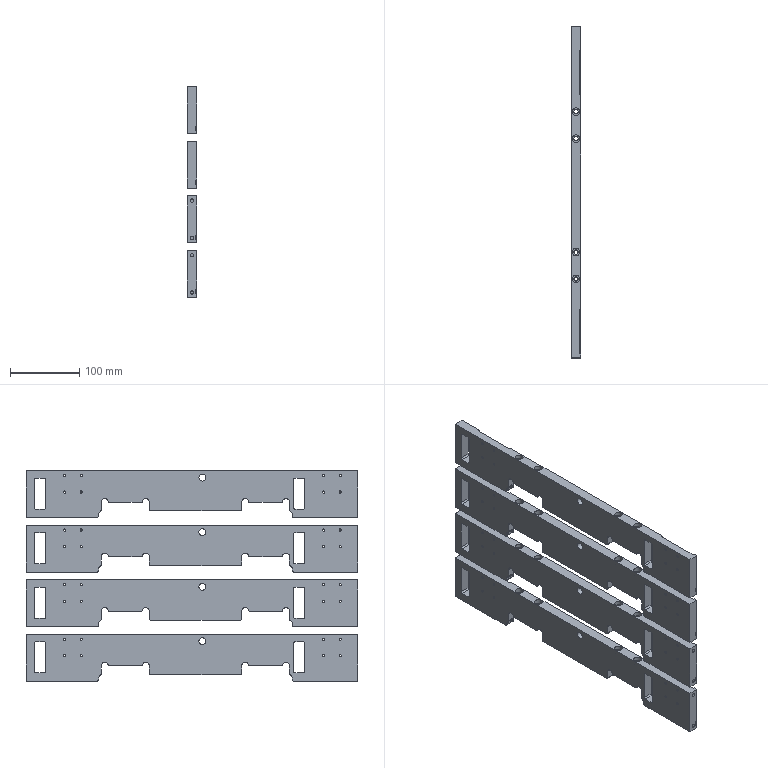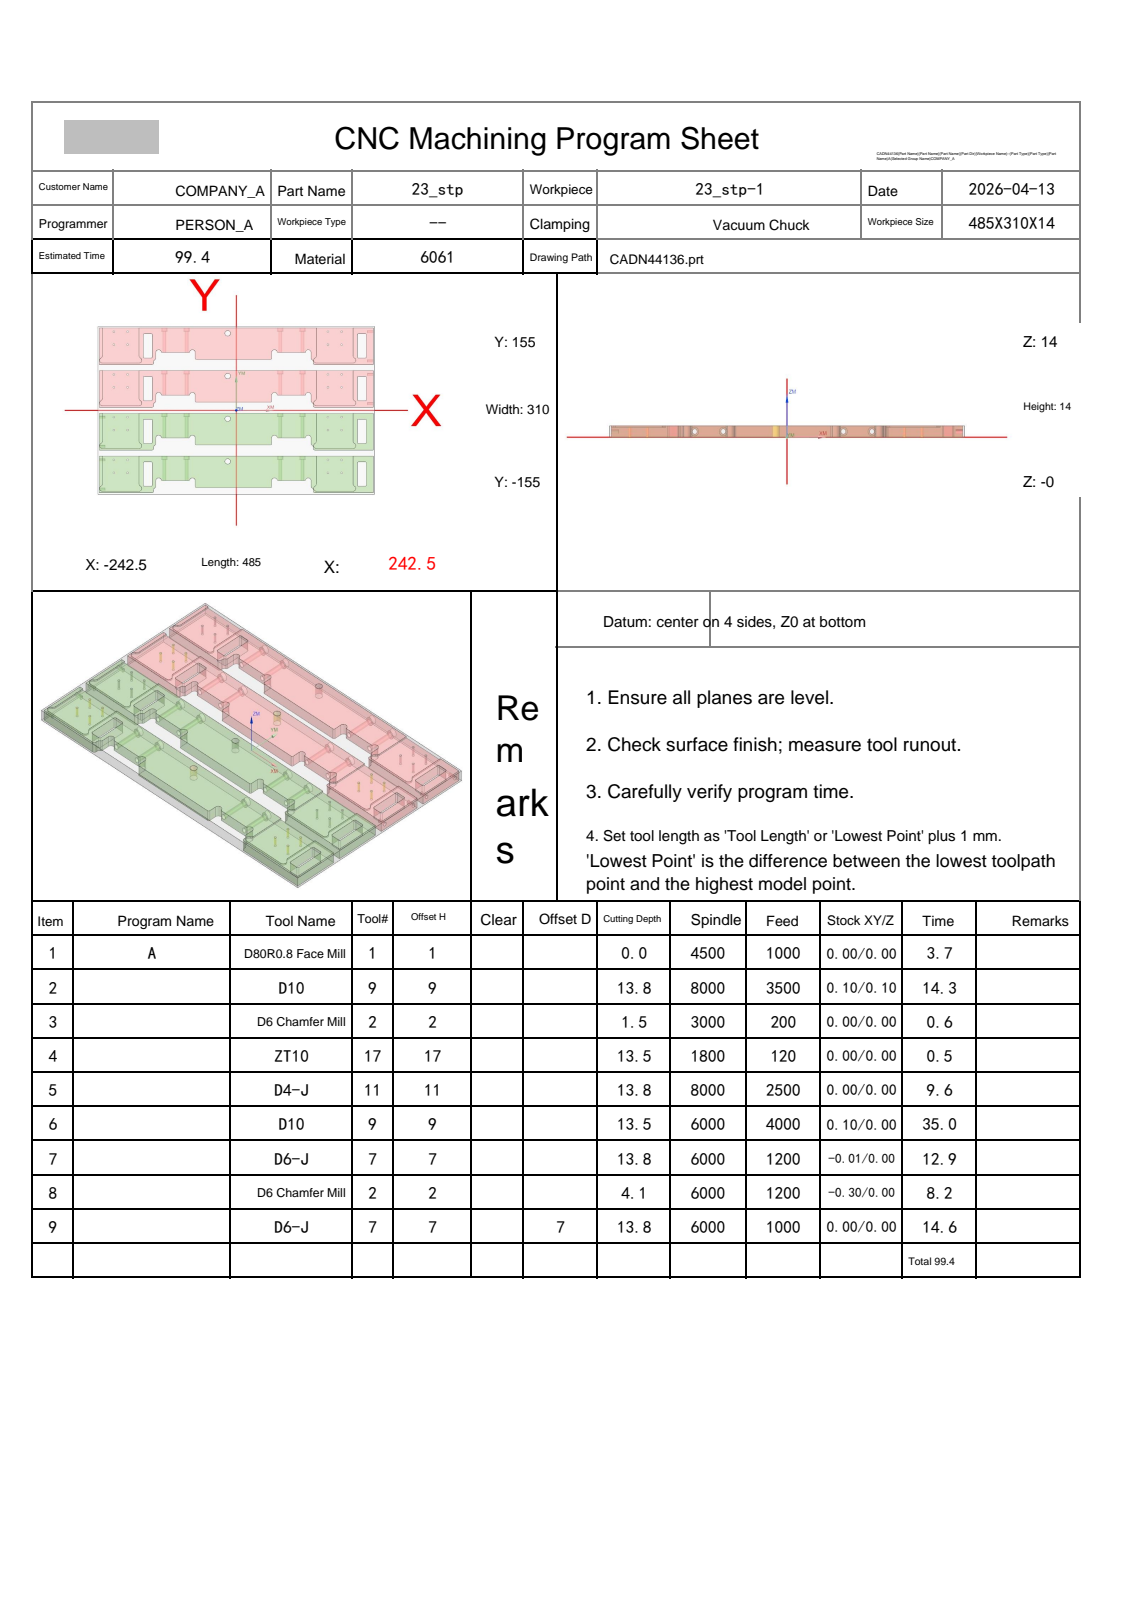NC program | NX | posted by the shop | part box 14 x 480 x 305 mm
Lines 49519 to 51894 of 51894, first 2165 of 2376 lines:
N7 T07 M06
(D6-J  D=6. R=0. H=07 ce=0.30 di=0.00)
G00 G90 G54 X143.75 Y-98.104 M03 S6000
G43 H07 Z34.
M08
Z13.5
G01 Y-83.9 Z13.004 F1200.
X172.5 Z12.
X201.25
Y-135.84
G03 X205.375 Y-142.984 I8.25 J0.0
G02 X206.25 Y-144.5 I-.875 J-1.516
X204.5 Y-146.25 I-1.75 J0.0
G01 X140.5
G02 X138.75 Y-144.5 I0.0 J1.75
X139.625 Y-142.984 I1.75 J0.0
G03 X143.75 Y-135.84 I-4.125 J7.145
G01 Y-83.9
X172.5
Y-88.1
X197.05
Y-135.84
G03 X198.709 Y-142.05 I12.45 J0.0
G01 X146.291
G03 X147.95 Y-135.84 I-10.791 J6.21
G01 Y-88.1
X172.5
Y-92.3
X192.85
Y-135.84
G03 X192.972 Y-137.85 I16.65 J0.0
G01 X152.028
G03 X152.15 Y-135.84 I-16.528 J2.01
G01 Y-92.3
X172.5
Y-96.5
X188.65
Y-133.65
X156.35
Y-96.5
X172.5
Y-100.7
X184.45
Y-129.45
X160.55
Y-100.7
X172.5
Y-104.9
X180.25
Y-125.25
X164.75
Y-104.9
X172.5
Y-109.1
X176.05
Y-121.05
X168.95
Y-109.1
X172.5
Y-111.8
X173.35
Y-118.35
X171.65
Y-111.8
X172.5
X173.
Y-108.2
Z12.5
G00 Z34.
X143.75 Y-19.104
Z13.5
G01 Y-4.9 Z13.004
X172.5 Z12.
X201.25
Y-56.84
G03 X205.375 Y-63.984 I8.25 J0.0
G02 X206.25 Y-65.5 I-.875 J-1.516
X204.5 Y-67.25 I-1.75 J0.0
G01 X140.5
G02 X138.75 Y-65.5 I0.0 J1.75
X139.625 Y-63.984 I1.75 J0.0
G03 X143.75 Y-56.84 I-4.125 J7.145
G01 Y-4.9
X172.5
Y-9.1
X197.05
Y-56.84
G03 X198.709 Y-63.05 I12.45 J0.0
G01 X146.291
G03 X147.95 Y-56.84 I-10.791 J6.21
G01 Y-9.1
X172.5
Y-13.3
X192.85
Y-56.84
G03 X192.972 Y-58.85 I16.65 J0.0
G01 X152.028
G03 X152.15 Y-56.84 I-16.528 J2.01
G01 Y-13.3
X172.5
Y-17.5
X188.65
Y-54.65
X156.35
Y-17.5
X172.5
Y-21.7
X184.45
Y-50.45
X160.55
Y-21.7
X172.5
Y-25.9
X180.25
Y-46.25
X164.75
Y-25.9
X172.5
Y-30.1
X176.05
Y-42.05
X168.95
Y-30.1
X172.5
Y-32.8
X173.35
Y-39.35
X171.65
Y-32.8
X172.5
X173.
Y-29.2
Z12.5
G00 Z34.
X143.75 Y59.896
Z13.5
G01 Y74.1 Z13.004
X172.5 Z12.
X201.25
Y22.16
G03 X205.375 Y15.016 I8.25 J0.0
G02 X206.25 Y13.5 I-.875 J-1.516
X204.5 Y11.75 I-1.75 J0.0
G01 X140.5
G02 X138.75 Y13.5 I0.0 J1.75
X139.625 Y15.016 I1.75 J0.0
G03 X143.75 Y22.16 I-4.125 J7.145
G01 Y74.1
X172.5
Y69.9
X197.05
Y22.16
G03 X198.709 Y15.95 I12.45 J0.0
G01 X146.291
G03 X147.95 Y22.16 I-10.791 J6.21
G01 Y69.9
X172.5
Y65.7
X192.85
Y22.16
G03 X192.972 Y20.15 I16.65 J0.0
G01 X152.028
G03 X152.15 Y22.16 I-16.528 J2.01
G01 Y65.7
X172.5
Y61.5
X188.65
Y24.35
X156.35
Y61.5
X172.5
Y57.3
X184.45
Y28.55
X160.55
Y57.3
X172.5
Y53.1
X180.25
Y32.75
X164.75
Y53.1
X172.5
Y48.9
X176.05
Y36.95
X168.95
Y48.9
X172.5
Y46.2
X173.35
Y39.65
X171.65
Y46.2
X172.5
X173.
Y49.8
Z12.5
G00 Z34.
X172.5 Y158.5
Z12.5
G01 Z12.
Y153.1
X201.25
Y101.16
G03 X205.375 Y94.016 I8.25 J0.0
G02 X206.25 Y92.5 I-.875 J-1.516
X204.5 Y90.75 I-1.75 J0.0
G01 X140.5
G02 X138.75 Y92.5 I0.0 J1.75
X139.625 Y94.016 I1.75 J0.0
G03 X143.75 Y101.16 I-4.125 J7.145
G01 Y153.1
X172.5
Y148.9
X197.05
Y101.16
G03 X198.709 Y94.95 I12.45 J0.0
G01 X146.291
G03 X147.95 Y101.16 I-10.791 J6.21
G01 Y148.9
X172.5
Y144.7
X192.85
Y101.16
G03 X192.972 Y99.15 I16.65 J0.0
G01 X152.028
G03 X152.15 Y101.16 I-16.528 J2.01
G01 Y144.7
X172.5
Y140.5
X188.65
Y103.35
X156.35
Y140.5
X172.5
Y136.3
X184.45
Y107.55
X160.55
Y136.3
X172.5
Y132.1
X180.25
Y111.75
X164.75
Y132.1
X172.5
Y127.9
X176.05
Y115.95
X168.95
Y127.9
X172.5
Y125.2
X173.35
Y118.65
X171.65
Y125.2
X172.5
X173.
Y128.8
Z12.5
G00 Z34.
X-202.5 Y158.5
Z12.5
G01 Z12.
Y153.1
X-173.75
Y101.16
G03 X-169.625 Y94.016 I8.25 J0.0
G02 X-168.75 Y92.5 I-.875 J-1.516
X-170.5 Y90.75 I-1.75 J0.0
G01 X-234.5
G02 X-236.25 Y92.5 I0.0 J1.75
X-235.375 Y94.016 I1.75 J0.0
G03 X-231.25 Y101.16 I-4.125 J7.145
G01 Y153.1
X-202.5
Y148.9
X-177.95
Y101.16
G03 X-176.291 Y94.95 I12.45 J0.0
G01 X-228.709
G03 X-227.05 Y101.16 I-10.791 J6.21
G01 Y148.9
X-202.5
Y144.7
X-182.15
Y101.16
G03 X-182.028 Y99.15 I16.65 J0.0
G01 X-222.972
G03 X-222.85 Y101.16 I-16.528 J2.01
G01 Y144.7
X-202.5
Y140.5
X-186.35
Y103.35
X-218.65
Y140.5
X-202.5
Y136.3
X-190.55
Y107.55
X-214.45
Y136.3
X-202.5
Y132.1
X-194.75
Y111.75
X-210.25
Y132.1
X-202.5
Y127.9
X-198.95
Y115.95
X-206.05
Y127.9
X-202.5
Y125.2
X-201.65
Y118.65
X-203.35
Y125.2
X-202.5
X-202.
Y128.8
Z12.5
G00 Z34.
X-231.25 Y59.896
Z13.5
G01 Y74.1 Z13.004
X-202.5 Z12.
X-173.75
Y22.16
G03 X-169.625 Y15.016 I8.25 J0.0
G02 X-168.75 Y13.5 I-.875 J-1.516
X-170.5 Y11.75 I-1.75 J0.0
G01 X-234.5
G02 X-236.25 Y13.5 I0.0 J1.75
X-235.375 Y15.016 I1.75 J0.0
G03 X-231.25 Y22.16 I-4.125 J7.145
G01 Y74.1
X-202.5
Y69.9
X-177.95
Y22.16
G03 X-176.291 Y15.95 I12.45 J0.0
G01 X-228.709
G03 X-227.05 Y22.16 I-10.791 J6.21
G01 Y69.9
X-202.5
Y65.7
X-182.15
Y22.16
G03 X-182.028 Y20.15 I16.65 J0.0
G01 X-222.972
G03 X-222.85 Y22.16 I-16.528 J2.01
G01 Y65.7
X-202.5
Y61.5
X-186.35
Y24.35
X-218.65
Y61.5
X-202.5
Y57.3
X-190.55
Y28.55
X-214.45
Y57.3
X-202.5
Y53.1
X-194.75
Y32.75
X-210.25
Y53.1
X-202.5
Y48.9
X-198.95
Y36.95
X-206.05
Y48.9
X-202.5
Y46.2
X-201.65
Y39.65
X-203.35
Y46.2
X-202.5
X-202.
Y49.8
Z12.5
G00 Z34.
X-231.25 Y-19.104
Z13.5
G01 Y-4.9 Z13.004
X-202.5 Z12.
X-173.75
Y-56.84
G03 X-169.625 Y-63.984 I8.25 J0.0
G02 X-168.75 Y-65.5 I-.875 J-1.516
X-170.5 Y-67.25 I-1.75 J0.0
G01 X-234.5
G02 X-236.25 Y-65.5 I0.0 J1.75
X-235.375 Y-63.984 I1.75 J0.0
G03 X-231.25 Y-56.84 I-4.125 J7.145
G01 Y-4.9
X-202.5
Y-9.1
X-177.95
Y-56.84
G03 X-176.291 Y-63.05 I12.45 J0.0
G01 X-228.709
G03 X-227.05 Y-56.84 I-10.791 J6.21
G01 Y-9.1
X-202.5
Y-13.3
X-182.15
Y-56.84
G03 X-182.028 Y-58.85 I16.65 J0.0
G01 X-222.972
G03 X-222.85 Y-56.84 I-16.528 J2.01
G01 Y-13.3
X-202.5
Y-17.5
X-186.35
Y-54.65
X-218.65
Y-17.5
X-202.5
Y-21.7
X-190.55
Y-50.45
X-214.45
Y-21.7
X-202.5
Y-25.9
X-194.75
Y-46.25
X-210.25
Y-25.9
X-202.5
Y-30.1
X-198.95
Y-42.05
X-206.05
Y-30.1
X-202.5
Y-32.8
X-201.65
Y-39.35
X-203.35
Y-32.8
X-202.5
X-202.
Y-29.2
Z12.5
G00 Z34.
X-231.25 Y-98.104
Z13.5
G01 Y-83.9 Z13.004
X-202.5 Z12.
X-173.75
Y-135.84
G03 X-169.625 Y-142.984 I8.25 J0.0
G02 X-168.75 Y-144.5 I-.875 J-1.516
X-170.5 Y-146.25 I-1.75 J0.0
G01 X-234.5
G02 X-236.25 Y-144.5 I0.0 J1.75
X-235.375 Y-142.984 I1.75 J0.0
G03 X-231.25 Y-135.84 I-4.125 J7.145
G01 Y-83.9
X-202.5
Y-88.1
X-177.95
Y-135.84
G03 X-176.291 Y-142.05 I12.45 J0.0
G01 X-228.709
G03 X-227.05 Y-135.84 I-10.791 J6.21
G01 Y-88.1
X-202.5
Y-92.3
X-182.15
Y-135.84
G03 X-182.028 Y-137.85 I16.65 J0.0
G01 X-222.972
G03 X-222.85 Y-135.84 I-16.528 J2.01
G01 Y-92.3
X-202.5
Y-96.5
X-186.35
Y-133.65
X-218.65
Y-96.5
X-202.5
Y-100.7
X-190.55
Y-129.45
X-214.45
Y-100.7
X-202.5
Y-104.9
X-194.75
Y-125.25
X-210.25
Y-104.9
X-202.5
Y-109.1
X-198.95
Y-121.05
X-206.05
Y-109.1
X-202.5
Y-111.8
X-201.65
Y-118.35
X-203.35
Y-111.8
X-202.5
X-202.
Y-108.2
Z12.5
G00 Z34.
G00 G90 X-230.46 Y-80.8 M03 S6000
Z34.
Z12.505
G01 Z12.005 F1200.
G41 D07
X-230.56
G03 X-231.56 Y-81.8 I0.0 J-1.
G01 Y-135.84
G02 X-235.53 Y-142.716 I-7.94 J0.0
G03 X-236.56 Y-144.5 I1.03 J-1.784
X-234.5 Y-146.56 I2.06 J0.0
G01 X-170.5
G03 X-168.44 Y-144.5 I0.0 J2.06
X-169.47 Y-142.716 I-2.06 J0.0
G02 X-173.44 Y-135.84 I3.97 J6.876
G01 Y-81.8
G03 X-174.44 Y-80.8 I-1. J0.0
G01 G40 X-174.54
Z12.505
G00 Z34.
X-230.46 Y-1.8
Z12.505
G01 Z12.005
G41 D07
X-230.56
G03 X-231.56 Y-2.8 I0.0 J-1.
G01 Y-56.84
G02 X-235.53 Y-63.716 I-7.94 J0.0
G03 X-236.56 Y-65.5 I1.03 J-1.784
X-234.5 Y-67.56 I2.06 J0.0
G01 X-170.5
G03 X-168.44 Y-65.5 I0.0 J2.06
X-169.47 Y-63.716 I-2.06 J0.0
G02 X-173.44 Y-56.84 I3.97 J6.876
G01 Y-2.8
G03 X-174.44 Y-1.8 I-1. J0.0
G01 G40 X-174.54
Z12.505
G00 Z34.
X-230.46 Y77.2
Z12.505
G01 Z12.005
G41 D07
X-230.56
G03 X-231.56 Y76.2 I0.0 J-1.
G01 Y22.16
G02 X-235.53 Y15.284 I-7.94 J0.0
G03 X-236.56 Y13.5 I1.03 J-1.784
X-234.5 Y11.44 I2.06 J0.0
G01 X-170.5
G03 X-168.44 Y13.5 I0.0 J2.06
X-169.47 Y15.284 I-2.06 J0.0
G02 X-173.44 Y22.16 I3.97 J6.876
G01 Y76.2
G03 X-174.44 Y77.2 I-1. J0.0
G01 G40 X-174.54
Z12.505
G00 Z34.
X-230.46 Y156.2
Z12.505
G01 Z12.005
G41 D07
X-230.56
G03 X-231.56 Y155.2 I0.0 J-1.
G01 Y101.16
G02 X-235.53 Y94.284 I-7.94 J0.0
G03 X-236.56 Y92.5 I1.03 J-1.784
X-234.5 Y90.44 I2.06 J0.0
G01 X-170.5
G03 X-168.44 Y92.5 I0.0 J2.06
X-169.47 Y94.284 I-2.06 J0.0
G02 X-173.44 Y101.16 I3.97 J6.876
G01 Y155.2
G03 X-174.44 Y156.2 I-1. J0.0
G01 G40 X-174.54
Z12.505
G00 Z34.
X144.54
Z12.505
G01 Z12.005
G41 D07
X144.44
G03 X143.44 Y155.2 I0.0 J-1.
G01 Y101.16
G02 X139.47 Y94.284 I-7.94 J0.0
G03 X138.44 Y92.5 I1.03 J-1.784
X140.5 Y90.44 I2.06 J0.0
G01 X204.5
G03 X206.56 Y92.5 I0.0 J2.06
X205.53 Y94.284 I-2.06 J0.0
G02 X201.56 Y101.16 I3.97 J6.876
G01 Y155.2
G03 X200.56 Y156.2 I-1. J0.0
G01 G40 X200.46
Z12.505
G00 Z34.
X144.54 Y77.2
Z12.505
G01 Z12.005
G41 D07
X144.44
G03 X143.44 Y76.2 I0.0 J-1.
G01 Y22.16
G02 X139.47 Y15.284 I-7.94 J0.0
G03 X138.44 Y13.5 I1.03 J-1.784
X140.5 Y11.44 I2.06 J0.0
G01 X204.5
G03 X206.56 Y13.5 I0.0 J2.06
X205.53 Y15.284 I-2.06 J0.0
G02 X201.56 Y22.16 I3.97 J6.876
G01 Y76.2
G03 X200.56 Y77.2 I-1. J0.0
G01 G40 X200.46
Z12.505
G00 Z34.
X144.54 Y-1.8
Z12.505
G01 Z12.005
G41 D07
X144.44
G03 X143.44 Y-2.8 I0.0 J-1.
G01 Y-56.84
G02 X139.47 Y-63.716 I-7.94 J0.0
G03 X138.44 Y-65.5 I1.03 J-1.784
X140.5 Y-67.56 I2.06 J0.0
G01 X204.5
G03 X206.56 Y-65.5 I0.0 J2.06
X205.53 Y-63.716 I-2.06 J0.0
G02 X201.56 Y-56.84 I3.97 J6.876
G01 Y-2.8
G03 X200.56 Y-1.8 I-1. J0.0
G01 G40 X200.46
Z12.505
G00 Z34.
X144.54 Y-80.8
Z12.505
G01 Z12.005
G41 D07
X144.44
G03 X143.44 Y-81.8 I0.0 J-1.
G01 Y-135.84
G02 X139.47 Y-142.716 I-7.94 J0.0
G03 X138.44 Y-144.5 I1.03 J-1.784
X140.5 Y-146.56 I2.06 J0.0
G01 X204.5
G03 X206.56 Y-144.5 I0.0 J2.06
X205.53 Y-142.716 I-2.06 J0.0
G02 X201.56 Y-135.84 I3.97 J6.876
G01 Y-81.8
G03 X200.56 Y-80.8 I-1. J0.0
G01 G40 X200.46
Z12.505
G00 Z34.
G00 G90 X-159.75 Y119.45 M03 S6000
Z34.
Z9.9
G01 Z9.4 F600.
G41 D07
X-159.8
G03 X-160. Y119.25 I0.0 J-.2
G01 Y99.75
X-150.
Y138.75
X-160.
Y119.25
Y118.75
G03 X-159.8 Y118.55 I.2 J0.0
G01 G40 X-159.75
Z9.9
G00 Z15.
Y119.45
Z5.3
G01 Z4.8
G41 D07
X-159.8
G03 X-160. Y119.25 I0.0 J-.2
G01 Y99.75
X-150.
Y138.75
X-160.
Y119.25
Y118.75
G03 X-159.8 Y118.55 I.2 J0.0
G01 G40 X-159.75
Z5.3
G00 Z10.4
Y119.45
Z.7
G01 Z.2
G41 D07
X-159.8
G03 X-160. Y119.25 I0.0 J-.2
G01 Y99.75
X-150.
Y138.75
X-160.
Y119.25
Y118.75
G03 X-159.8 Y118.55 I.2 J0.0
G01 G40 X-159.75
Z.7
G00 Z34.
Y40.45
Z9.9
G01 Z9.4
G41 D07
X-159.8
G03 X-160. Y40.25 I0.0 J-.2
G01 Y20.75
X-150.
Y59.75
X-160.
Y40.25
Y39.75
G03 X-159.8 Y39.55 I.2 J0.0
G01 G40 X-159.75
Z9.9
G00 Z15.
Y40.45
Z5.3
G01 Z4.8
G41 D07
X-159.8
G03 X-160. Y40.25 I0.0 J-.2
G01 Y20.75
X-150.
Y59.75
X-160.
Y40.25
Y39.75
G03 X-159.8 Y39.55 I.2 J0.0
G01 G40 X-159.75
Z5.3
G00 Z10.4
Y40.45
Z.7
G01 Z.2
G41 D07
X-159.8
G03 X-160. Y40.25 I0.0 J-.2
G01 Y20.75
X-150.
Y59.75
X-160.
Y40.25
Y39.75
G03 X-159.8 Y39.55 I.2 J0.0
G01 G40 X-159.75
Z.7
G00 Z34.
Y-38.55
Z9.9
G01 Z9.4
G41 D07
X-159.8
G03 X-160. Y-38.75 I0.0 J-.2
G01 Y-58.25
X-150.
Y-19.25
X-160.
Y-38.75
Y-39.25
G03 X-159.8 Y-39.45 I.2 J0.0
G01 G40 X-159.75
Z9.9
G00 Z15.
Y-38.55
Z5.3
G01 Z4.8
G41 D07
X-159.8
G03 X-160. Y-38.75 I0.0 J-.2
G01 Y-58.25
X-150.
Y-19.25
X-160.
Y-38.75
Y-39.25
G03 X-159.8 Y-39.45 I.2 J0.0
G01 G40 X-159.75
Z5.3
G00 Z10.4
Y-38.55
Z.7
G01 Z.2
G41 D07
X-159.8
G03 X-160. Y-38.75 I0.0 J-.2
G01 Y-58.25
X-150.
Y-19.25
X-160.
Y-38.75
Y-39.25
G03 X-159.8 Y-39.45 I.2 J0.0
G01 G40 X-159.75
Z.7
G00 Z34.
Y-117.55
Z9.9
G01 Z9.4
G41 D07
X-159.8
G03 X-160. Y-117.75 I0.0 J-.2
G01 Y-137.25
X-150.
Y-98.25
X-160.
Y-117.75
Y-118.25
G03 X-159.8 Y-118.45 I.2 J0.0
G01 G40 X-159.75
Z9.9
G00 Z15.
Y-117.55
Z5.3
G01 Z4.8
G41 D07
X-159.8
G03 X-160. Y-117.75 I0.0 J-.2
G01 Y-137.25
X-150.
Y-98.25
X-160.
Y-117.75
Y-118.25
G03 X-159.8 Y-118.45 I.2 J0.0
G01 G40 X-159.75
Z5.3
G00 Z10.4
Y-117.55
Z.7
G01 Z.2
G41 D07
X-159.8
G03 X-160. Y-117.75 I0.0 J-.2
G01 Y-137.25
X-150.
Y-98.25
X-160.
Y-117.75
Y-118.25
G03 X-159.8 Y-118.45 I.2 J0.0
G01 G40 X-159.75
Z.7
G00 Z34.
X224.75 Y-117.95
Z9.9
G01 Z9.4
G41 D07
X224.8
G03 X225. Y-117.75 I0.0 J.2
G01 Y-98.25
X215.
Y-137.25
X225.
Y-117.75
Y-117.25
G03 X224.8 Y-117.05 I-.2 J0.0
G01 G40 X224.75
Z9.9
G00 Z15.
Y-117.95
Z5.3
G01 Z4.8
G41 D07
X224.8
G03 X225. Y-117.75 I0.0 J.2
G01 Y-98.25
X215.
Y-137.25
X225.
Y-117.75
Y-117.25
G03 X224.8 Y-117.05 I-.2 J0.0
G01 G40 X224.75
Z5.3
G00 Z10.4
Y-117.95
Z.7
G01 Z.2
G41 D07
X224.8
G03 X225. Y-117.75 I0.0 J.2
G01 Y-98.25
X215.
Y-137.25
X225.
Y-117.75
Y-117.25
G03 X224.8 Y-117.05 I-.2 J0.0
G01 G40 X224.75
Z.7
G00 Z34.
Y-38.95
Z9.9
G01 Z9.4
G41 D07
X224.8
G03 X225. Y-38.75 I0.0 J.2
G01 Y-19.25
X215.
Y-58.25
X225.
Y-38.75
Y-38.25
G03 X224.8 Y-38.05 I-.2 J0.0
G01 G40 X224.75
Z9.9
G00 Z15.
Y-38.95
Z5.3
G01 Z4.8
G41 D07
X224.8
G03 X225. Y-38.75 I0.0 J.2
G01 Y-19.25
X215.
Y-58.25
X225.
Y-38.75
Y-38.25
G03 X224.8 Y-38.05 I-.2 J0.0
G01 G40 X224.75
Z5.3
G00 Z10.4
Y-38.95
Z.7
G01 Z.2
G41 D07
X224.8
G03 X225. Y-38.75 I0.0 J.2
G01 Y-19.25
X215.
Y-58.25
X225.
Y-38.75
Y-38.25
G03 X224.8 Y-38.05 I-.2 J0.0
G01 G40 X224.75
Z.7
G00 Z34.
Y40.05
Z9.9
G01 Z9.4
G41 D07
X224.8
G03 X225. Y40.25 I0.0 J.2
G01 Y59.75
X215.
Y20.75
X225.
Y40.25
Y40.75
G03 X224.8 Y40.95 I-.2 J0.0
G01 G40 X224.75
Z9.9
G00 Z15.
Y40.05
Z5.3
G01 Z4.8
G41 D07
X224.8
G03 X225. Y40.25 I0.0 J.2
G01 Y59.75
X215.
Y20.75
X225.
Y40.25
Y40.75
G03 X224.8 Y40.95 I-.2 J0.0
G01 G40 X224.75
Z5.3
G00 Z10.4
Y40.05
Z.7
G01 Z.2
G41 D07
X224.8
G03 X225. Y40.25 I0.0 J.2
G01 Y59.75
X215.
Y20.75
X225.
Y40.25
Y40.75
G03 X224.8 Y40.95 I-.2 J0.0
G01 G40 X224.75
Z.7
G00 Z34.
Y119.05
Z9.9
G01 Z9.4
G41 D07
X224.8
G03 X225. Y119.25 I0.0 J.2
G01 Y138.75
X215.
Y99.75
X225.
Y119.25
Y119.75
G03 X224.8 Y119.95 I-.2 J0.0
G01 G40 X224.75
Z9.9
G00 Z15.
Y119.05
Z5.3
G01 Z4.8
G41 D07
X224.8
G03 X225. Y119.25 I0.0 J.2
G01 Y138.75
X215.
Y99.75
X225.
Y119.25
Y119.75
G03 X224.8 Y119.95 I-.2 J0.0
G01 G40 X224.75
Z5.3
G00 Z10.4
Y119.05
Z.7
G01 Z.2
G41 D07
X224.8
G03 X225. Y119.25 I0.0 J.2
G01 Y138.75
X215.
Y99.75
X225.
Y119.25
Y119.75
G03 X224.8 Y119.95 I-.2 J0.0
G01 G40 X224.75
Z.7
G00 Z34.
G91 G28 Z0.0
M05
M09
G91 G28 Z0.0
M01
N8 T02 M06
(D6 Chamfer Mill  D=6. R=0. H=02 ce=0.00 di=0.00)
G00 G90 G54 X-15.25 Y-3.372 M03 S6000
G43 H02 Z34.
M08
Z16.099
G01 Z12.5 F1200.
G03 X-15.33 Y-3.672 I.52 J-.3
X-15.03 Y-4.192 I.6 J0.0
G01 X-15. Y-4.2
X140.45
G02 X141.75 Y-5.5 I0.0 J-1.3
G01 Y-56.84
G02 X138.625 Y-62.252 I-6.25 J0.0
G03 X136.75 Y-65.5 I1.875 J-3.248
X138.915 Y-68.899 I3.75 J0.0
G01 X139.424 Y-69.092
X139.957 Y-69.21
X140.5 Y-69.25
X204.5
G03 X208.25 Y-65.5 I0.0 J3.75
X207.851 Y-63.817 I-3.75 J0.0
G01 X207.572 Y-63.349
X207.228 Y-62.927
X206.826 Y-62.558
X206.375 Y-62.252
G02 X203.25 Y-56.84 I3.125 J5.413
G01 Y-5.5
G02 X204.55 Y-4.2 I1.3 J0.0
G01 X240.
G02 X241.3 Y-5.5 I0.0 J-1.3
G01 Y-73.5
G02 X240. Y-74.8 I-1.3 J0.0
G01 X138.
G02 X133.7 Y-70.5 I0.0 J4.3
G01 Y-68.499
G03 X131.639 Y-65.181 I-3.7 J0.0
G02 X129.8 Y-62.222 I1.461 J2.959
G01 Y-50.9
G03 X126.1 Y-47.2 I-3.7 J0.0
X122.5 Y-50.046 I0.0 J-3.7
G02 X119.775 Y-52.2 I-2.724 J.646
G01 X73.225
G02 X70.5 Y-50.046 I0.0 J2.8
G03 X66.9 Y-47.2 I-3.6 J-.854
X63.2 Y-50.9 I0.0 J-3.7
G01 Y-61.9
G02 X59.9 Y-65.2 I-3.3 J0.0
G01 X-69.9
G02 X-73.2 Y-61.9 I0.0 J3.3
G01 Y-50.9
G03 X-76.9 Y-47.2 I-3.7 J0.0
X-80.5 Y-50.046 I0.0 J-3.7
G02 X-83.225 Y-52.2 I-2.724 J.646
G01 X-129.775
G02 X-132.5 Y-50.046 I0.0 J2.8
G03 X-136.1 Y-47.2 I-3.6 J-.854
X-139.8 Y-50.9 I0.0 J-3.7
G01 Y-62.222
G02 X-141.639 Y-65.181 I-3.3 J0.0
G03 X-143.7 Y-68.499 I1.639 J-3.317
G01 Y-70.5
G02 X-148. Y-74.8 I-4.3 J0.0
G01 X-240.
G02 X-241.3 Y-73.5 I0.0 J1.3
G01 Y-5.5
G02 X-240. Y-4.2 I1.3 J0.0
G01 X-234.55
G02 X-233.25 Y-5.5 I0.0 J-1.3
G01 Y-56.84
G02 X-236.375 Y-62.252 I-6.25 J0.0
G03 X-238.25 Y-65.5 I1.875 J-3.248
X-236.561 Y-68.633 I3.75 J0.0
G01 X-236.085 Y-68.899
X-235.576 Y-69.092
X-235.043 Y-69.21
X-234.5 Y-69.25
X-170.5
G03 X-166.75 Y-65.5 I0.0 J3.75
X-167.149 Y-63.817 I-3.75 J0.0
G01 X-167.428 Y-63.349
X-167.772 Y-62.927
X-168.174 Y-62.558
X-168.625 Y-62.252
G02 X-171.75 Y-56.84 I3.125 J5.413
G01 Y-5.5
G02 X-170.45 Y-4.2 I1.3 J0.0
G01 X-15.
X-14.97 Y-4.192
G03 X-14.67 Y-3.672 I-.3 J.52
X-14.75 Y-3.372 I-.6 J0.0
G01 Z16.099
G00 Z34.
X214.128 Y-38.5
Z16.099
G01 Z12.5
G03 X213.828 Y-38.42 I-.3 J-.52
X213.308 Y-38.72 I0.0 J-.6
G01 X213.3 Y-38.75
Y-59.25
G03 X214. Y-59.95 I.7 J0.0
G01 X226.
G03 X226.7 Y-59.25 I0.0 J.7
G01 Y-18.25
G03 X226. Y-17.55 I-.7 J0.0
G01 X214.
G03 X213.3 Y-18.25 I0.0 J-.7
G01 Y-38.75
X213.308 Y-38.78
G03 X213.828 Y-39.08 I.52 J.3
X214.128 Y-39. I0.0 J.6
G01 Z16.099
G00 Z34.
X-149.128
Z16.099
G01 Z12.5
G03 X-148.828 Y-39.08 I.3 J.52
X-148.308 Y-38.78 I0.0 J.6
G01 X-148.3 Y-38.75
Y-18.25
G03 X-149. Y-17.55 I-.7 J0.0
G01 X-161.
G03 X-161.7 Y-18.25 I0.0 J-.7
G01 Y-59.25
G03 X-161. Y-59.95 I.7 J0.0
G01 X-149.
G03 X-148.3 Y-59.25 I0.0 J.7
G01 Y-38.75
X-148.308 Y-38.72
G03 X-148.828 Y-38.42 I-.52 J-.3
X-149.128 Y-38.5 I0.0 J-.6
G01 Z16.099
G00 Z34.
X-15.25 Y-82.372
Z16.099
G01 Z12.5
G03 X-15.33 Y-82.672 I.52 J-.3
X-15.03 Y-83.192 I.6 J0.0
G01 X-15. Y-83.2
X140.45
G02 X141.75 Y-84.5 I0.0 J-1.3
G01 Y-135.84
G02 X138.625 Y-141.252 I-6.25 J0.0
G03 X136.75 Y-144.5 I1.875 J-3.248
X138.915 Y-147.899 I3.75 J0.0
G01 X139.424 Y-148.092
X139.957 Y-148.21
X140.5 Y-148.25
X204.5
G03 X208.25 Y-144.5 I0.0 J3.75
X207.851 Y-142.817 I-3.75 J0.0
G01 X207.572 Y-142.349
X207.228 Y-141.927
X206.826 Y-141.558
X206.375 Y-141.252
G02 X203.25 Y-135.84 I3.125 J5.413
G01 Y-84.5
G02 X204.55 Y-83.2 I1.3 J0.0
G01 X240.
G02 X241.3 Y-84.5 I0.0 J-1.3
G01 Y-152.5
G02 X240. Y-153.8 I-1.3 J0.0
G01 X138.
G02 X133.7 Y-149.5 I0.0 J4.3
G01 Y-147.499
G03 X131.639 Y-144.181 I-3.7 J0.0
G02 X129.8 Y-141.222 I1.461 J2.959
G01 Y-129.9
G03 X126.1 Y-126.2 I-3.7 J0.0
X122.5 Y-129.046 I0.0 J-3.7
G02 X119.775 Y-131.2 I-2.724 J.646
G01 X73.225
G02 X70.5 Y-129.046 I0.0 J2.8
G03 X66.9 Y-126.2 I-3.6 J-.854
X63.2 Y-129.9 I0.0 J-3.7
G01 Y-140.9
G02 X59.9 Y-144.2 I-3.3 J0.0
G01 X-69.9
G02 X-73.2 Y-140.9 I0.0 J3.3
G01 Y-129.9
G03 X-76.9 Y-126.2 I-3.7 J0.0
X-80.5 Y-129.046 I0.0 J-3.7
G02 X-83.225 Y-131.2 I-2.724 J.646
G01 X-129.775
G02 X-132.5 Y-129.046 I0.0 J2.8
G03 X-136.1 Y-126.2 I-3.6 J-.854
X-139.8 Y-129.9 I0.0 J-3.7
G01 Y-141.222
G02 X-141.639 Y-144.181 I-3.3 J0.0
G03 X-143.7 Y-147.499 I1.639 J-3.317
G01 Y-149.5
G02 X-148. Y-153.8 I-4.3 J0.0
G01 X-240.
G02 X-241.3 Y-152.5 I0.0 J1.3
G01 Y-84.5
G02 X-240. Y-83.2 I1.3 J0.0
G01 X-234.55
G02 X-233.25 Y-84.5 I0.0 J-1.3
G01 Y-135.84
G02 X-236.375 Y-141.252 I-6.25 J0.0
G03 X-238.25 Y-144.5 I1.875 J-3.248
X-236.561 Y-147.633 I3.75 J0.0
G01 X-236.085 Y-147.899
X-235.576 Y-148.092
X-235.043 Y-148.21
X-234.5 Y-148.25
X-170.5
G03 X-166.75 Y-144.5 I0.0 J3.75
X-167.149 Y-142.817 I-3.75 J0.0
G01 X-167.428 Y-142.349
X-167.772 Y-141.927
X-168.174 Y-141.558
X-168.625 Y-141.252
G02 X-171.75 Y-135.84 I3.125 J5.413
G01 Y-84.5
G02 X-170.45 Y-83.2 I1.3 J0.0
G01 X-15.
X-14.97 Y-83.192
G03 X-14.67 Y-82.672 I-.3 J.52
X-14.75 Y-82.372 I-.6 J0.0
G01 Z16.099
G00 Z34.
X214.128 Y-117.5
Z16.099
G01 Z12.5
G03 X213.828 Y-117.42 I-.3 J-.52
X213.308 Y-117.72 I0.0 J-.6
G01 X213.3 Y-117.75
Y-138.25
G03 X214. Y-138.95 I.7 J0.0
G01 X226.
G03 X226.7 Y-138.25 I0.0 J.7
G01 Y-97.25
G03 X226. Y-96.55 I-.7 J0.0
G01 X214.
G03 X213.3 Y-97.25 I0.0 J-.7
G01 Y-117.75
X213.308 Y-117.78
G03 X213.828 Y-118.08 I.52 J.3
X214.128 Y-118. I0.0 J.6
G01 Z16.099
G00 Z34.
X-149.128
Z16.099
G01 Z12.5
G03 X-148.828 Y-118.08 I.3 J.52
X-148.308 Y-117.78 I0.0 J.6
G01 X-148.3 Y-117.75
Y-97.25
G03 X-149. Y-96.55 I-.7 J0.0
G01 X-161.
G03 X-161.7 Y-97.25 I0.0 J-.7
G01 Y-138.25
G03 X-161. Y-138.95 I.7 J0.0
G01 X-149.
G03 X-148.3 Y-138.25 I0.0 J.7
G01 Y-117.75
X-148.308 Y-117.72
G03 X-148.828 Y-117.42 I-.52 J-.3
X-149.128 Y-117.5 I0.0 J-.6
G01 Z16.099
G00 Z34.
X-15.25 Y75.628
Z16.099
G01 Z12.5
G03 X-15.33 Y75.328 I.52 J-.3
X-15.03 Y74.808 I.6 J0.0
G01 X-15. Y74.8
X140.45
G02 X141.75 Y73.5 I0.0 J-1.3
G01 Y22.16
G02 X138.625 Y16.748 I-6.25 J0.0
G03 X136.75 Y13.5 I1.875 J-3.248
X138.915 Y10.101 I3.75 J0.0
G01 X139.424 Y9.908
X139.957 Y9.79
X140.5 Y9.75
X204.5
G03 X208.25 Y13.5 I0.0 J3.75
X207.851 Y15.183 I-3.75 J0.0
G01 X207.572 Y15.651
X207.228 Y16.073
X206.826 Y16.442
X206.375 Y16.748
G02 X203.25 Y22.16 I3.125 J5.413
G01 Y73.5
G02 X204.55 Y74.8 I1.3 J0.0
G01 X240.
G02 X241.3 Y73.5 I0.0 J-1.3
G01 Y5.5
G02 X240. Y4.2 I-1.3 J0.0
G01 X138.
G02 X133.7 Y8.5 I0.0 J4.3
G01 Y10.501
G03 X131.639 Y13.819 I-3.7 J0.0
G02 X129.8 Y16.778 I1.461 J2.959
G01 Y28.1
G03 X126.1 Y31.8 I-3.7 J0.0
X122.4 Y28.1 I0.0 J-3.7
G02 X121.1 Y26.8 I-1.3 J0.0
G01 X71.9
G02 X70.6 Y28.1 I0.0 J1.3
G03 X66.9 Y31.8 I-3.7 J0.0
X63.2 Y28.1 I0.0 J-3.7
G01 Y17.1
G02 X59.9 Y13.8 I-3.3 J0.0
G01 X-69.9
G02 X-73.2 Y17.1 I0.0 J3.3
G01 Y28.1
G03 X-76.9 Y31.8 I-3.7 J0.0
X-80.6 Y28.1 I0.0 J-3.7
G02 X-81.9 Y26.8 I-1.3 J0.0
G01 X-131.1
G02 X-132.4 Y28.1 I0.0 J1.3
G03 X-136.1 Y31.8 I-3.7 J0.0
X-139.8 Y28.1 I0.0 J-3.7
G01 Y16.778
G02 X-141.639 Y13.819 I-3.3 J0.0
G03 X-143.7 Y10.501 I1.639 J-3.317
G01 Y8.5
G02 X-148. Y4.2 I-4.3 J0.0
G01 X-240.
G02 X-241.3 Y5.5 I0.0 J1.3
G01 Y73.5
G02 X-240. Y74.8 I1.3 J0.0
G01 X-234.55
G02 X-233.25 Y73.5 I0.0 J-1.3
G01 Y22.16
G02 X-236.375 Y16.748 I-6.25 J0.0
G03 X-238.25 Y13.5 I1.875 J-3.248
X-236.561 Y10.367 I3.75 J0.0
G01 X-236.085 Y10.101
X-235.576 Y9.908
X-235.043 Y9.79
X-234.5 Y9.75
X-170.5
G03 X-166.75 Y13.5 I0.0 J3.75
X-167.149 Y15.183 I-3.75 J0.0
G01 X-167.428 Y15.651
X-167.772 Y16.073
X-168.174 Y16.442
X-168.625 Y16.748
G02 X-171.75 Y22.16 I3.125 J5.413
G01 Y73.5
G02 X-170.45 Y74.8 I1.3 J0.0
G01 X-15.
X-14.97 Y74.808
G03 X-14.67 Y75.328 I-.3 J.52
X-14.75 Y75.628 I-.6 J0.0
G01 Z16.099
G00 Z34.
X-149.128 Y40.
Z16.099
G01 Z12.5
G03 X-148.828 Y39.92 I.3 J.52
X-148.308 Y40.22 I0.0 J.6
G01 X-148.3 Y40.25
Y60.75
G03 X-149. Y61.45 I-.7 J0.0
G01 X-161.
G03 X-161.7 Y60.75 I0.0 J-.7
G01 Y19.75
G03 X-161. Y19.05 I.7 J0.0
G01 X-149.
G03 X-148.3 Y19.75 I0.0 J.7
G01 Y40.25
X-148.308 Y40.28
G03 X-148.828 Y40.58 I-.52 J-.3
X-149.128 Y40.5 I0.0 J-.6
G01 Z16.099
G00 Z34.
X214.128
Z16.099
G01 Z12.5
G03 X213.828 Y40.58 I-.3 J-.52
X213.308 Y40.28 I0.0 J-.6
G01 X213.3 Y40.25
Y19.75
G03 X214. Y19.05 I.7 J0.0
G01 X226.
G03 X226.7 Y19.75 I0.0 J.7
G01 Y60.75
G03 X226. Y61.45 I-.7 J0.0
G01 X214.
G03 X213.3 Y60.75 I0.0 J-.7
G01 Y40.25
X213.308 Y40.22
G03 X213.828 Y39.92 I.52 J.3
X214.128 Y40. I0.0 J.6
G01 Z16.099
G00 Z34.
X-15.25 Y154.628
Z16.099
G01 Z12.5
G03 X-15.33 Y154.328 I.52 J-.3
X-15.03 Y153.808 I.6 J0.0
G01 X-15. Y153.8
X140.45
G02 X141.75 Y152.5 I0.0 J-1.3
G01 Y101.16
G02 X138.625 Y95.748 I-6.25 J0.0
G03 X136.75 Y92.5 I1.875 J-3.248
X138.915 Y89.101 I3.75 J0.0
G01 X139.424 Y88.908
X139.957 Y88.79
X140.5 Y88.75
X204.5
G03 X208.25 Y92.5 I0.0 J3.75
X207.851 Y94.183 I-3.75 J0.0
G01 X207.572 Y94.651
X207.228 Y95.073
X206.826 Y95.442
X206.375 Y95.748
G02 X203.25 Y101.16 I3.125 J5.413
G01 Y152.5
G02 X204.55 Y153.8 I1.3 J0.0
G01 X240.
G02 X241.3 Y152.5 I0.0 J-1.3
G01 Y84.5
G02 X240. Y83.2 I-1.3 J0.0
G01 X138.
G02 X133.7 Y87.5 I0.0 J4.3
G01 Y89.501
G03 X131.639 Y92.819 I-3.7 J0.0
G02 X129.8 Y95.778 I1.461 J2.959
G01 Y107.1
G03 X126.1 Y110.8 I-3.7 J0.0
X122.4 Y107.1 I0.0 J-3.7
G02 X121.1 Y105.8 I-1.3 J0.0
G01 X71.9
G02 X70.6 Y107.1 I0.0 J1.3
G03 X66.9 Y110.8 I-3.7 J0.0
X63.2 Y107.1 I0.0 J-3.7
G01 Y96.1
G02 X59.9 Y92.8 I-3.3 J0.0
G01 X-69.9
G02 X-73.2 Y96.1 I0.0 J3.3
G01 Y107.1
G03 X-76.9 Y110.8 I-3.7 J0.0
X-80.6 Y107.1 I0.0 J-3.7
G02 X-81.9 Y105.8 I-1.3 J0.0
G01 X-131.1
G02 X-132.4 Y107.1 I0.0 J1.3
G03 X-136.1 Y110.8 I-3.7 J0.0
X-139.8 Y107.1 I0.0 J-3.7
G01 Y95.778
G02 X-141.639 Y92.819 I-3.3 J0.0
G03 X-143.7 Y89.501 I1.639 J-3.317
G01 Y87.5
G02 X-148. Y83.2 I-4.3 J0.0
G01 X-240.
G02 X-241.3 Y84.5 I0.0 J1.3
G01 Y152.5
G02 X-240. Y153.8 I1.3 J0.0
G01 X-234.55
G02 X-233.25 Y152.5 I0.0 J-1.3
G01 Y101.16
G02 X-236.375 Y95.748 I-6.25 J0.0
G03 X-238.25 Y92.5 I1.875 J-3.248
X-236.561 Y89.367 I3.75 J0.0
G01 X-236.085 Y89.101
X-235.576 Y88.908
X-235.043 Y88.79
X-234.5 Y88.75
X-170.5
G03 X-166.75 Y92.5 I0.0 J3.75
X-167.149 Y94.183 I-3.75 J0.0
G01 X-167.428 Y94.651
X-167.772 Y95.073
X-168.174 Y95.442
X-168.625 Y95.748
G02 X-171.75 Y101.16 I3.125 J5.413
G01 Y152.5
G02 X-170.45 Y153.8 I1.3 J0.0
G01 X-15.
X-14.97 Y153.808
G03 X-14.67 Y154.328 I-.3 J.52
X-14.75 Y154.628 I-.6 J0.0
G01 Z16.099
G00 Z34.
X-149.128 Y119.
Z16.099
G01 Z12.5
G03 X-148.828 Y118.92 I.3 J.52
X-148.308 Y119.22 I0.0 J.6
G01 X-148.3 Y119.25
Y139.75
G03 X-149. Y140.45 I-.7 J0.0
G01 X-161.
G03 X-161.7 Y139.75 I0.0 J-.7
G01 Y98.75
G03 X-161. Y98.05 I.7 J0.0
G01 X-149.
G03 X-148.3 Y98.75 I0.0 J.7
G01 Y119.25
X-148.308 Y119.28
G03 X-148.828 Y119.58 I-.52 J-.3
X-149.128 Y119.5 I0.0 J-.6
G01 Z16.099
G00 Z34.
X214.128
Z16.099
G01 Z12.5
G03 X213.828 Y119.58 I-.3 J-.52
X213.308 Y119.28 I0.0 J-.6
G01 X213.3 Y119.25
Y98.75
G03 X214. Y98.05 I.7 J0.0
G01 X226.
G03 X226.7 Y98.75 I0.0 J.7
G01 Y139.75
G03 X226. Y140.45 I-.7 J0.0
G01 X214.
G03 X213.3 Y139.75 I0.0 J-.7
G01 Y119.25
X213.308 Y119.22
G03 X213.828 Y118.92 I.52 J.3
X214.128 Y119. I0.0 J.6
G01 Z16.099
G00 Z34.
X143.487 Y154.628
Z15.755
G01 Z10.5
G03 X143.406 Y154.328 I.52 J-.3
X143.706 Y153.808 I.6 J0.0
G01 X143.736 Y153.8
X201.264
X201.294 Y153.808
G03 X201.594 Y154.328 I-.3 J.52
X201.513 Y154.628 I-.6 J0.0
G01 Z15.755
G00 Z34.
X143.487 Y75.628
Z15.755
G01 Z10.5
G03 X143.406 Y75.328 I.52 J-.3
X143.706 Y74.808 I.6 J0.0
G01 X143.736 Y74.8
X201.264
X201.294 Y74.808
G03 X201.594 Y75.328 I-.3 J.52
X201.513 Y75.628 I-.6 J0.0
G01 Z15.755
G00 Z34.
X143.487 Y-3.372
Z15.755
G01 Z10.5
G03 X143.406 Y-3.672 I.52 J-.3
X143.706 Y-4.192 I.6 J0.0
G01 X143.736 Y-4.2
X201.264
X201.294 Y-4.192
G03 X201.594 Y-3.672 I-.3 J.52
X201.513 Y-3.372 I-.6 J0.0
G01 Z15.755
G00 Z34.
X143.487 Y-82.372
Z15.755
G01 Z10.5
G03 X143.406 Y-82.672 I.52 J-.3
X143.706 Y-83.192 I.6 J0.0
G01 X143.736 Y-83.2
X201.264
X201.294 Y-83.192
G03 X201.594 Y-82.672 I-.3 J.52
X201.513 Y-82.372 I-.6 J0.0
G01 Z15.755
G00 Z34.
X-231.513
Z15.755
G01 Z10.5
G03 X-231.594 Y-82.672 I.52 J-.3
X-231.294 Y-83.192 I.6 J0.0
G01 X-231.264 Y-83.2
X-173.736
X-173.706 Y-83.192
G03 X-173.406 Y-82.672 I-.3 J.52
X-173.487 Y-82.372 I-.6 J0.0
G01 Z15.755
G00 Z34.
X-231.513 Y-3.372
Z15.755
G01 Z10.5
G03 X-231.594 Y-3.672 I.52 J-.3
X-231.294 Y-4.192 I.6 J0.0
G01 X-231.264 Y-4.2
X-173.736
X-173.706 Y-4.192
G03 X-173.406 Y-3.672 I-.3 J.52
X-173.487 Y-3.372 I-.6 J0.0
G01 Z15.755
G00 Z34.
X-231.513 Y75.628
Z15.755
G01 Z10.5
G03 X-231.594 Y75.328 I.52 J-.3
X-231.294 Y74.808 I.6 J0.0
G01 X-231.264 Y74.8
X-173.736
X-173.706 Y74.808
G03 X-173.406 Y75.328 I-.3 J.52
X-173.487 Y75.628 I-.6 J0.0
G01 Z15.755
G00 Z34.
X-231.513 Y154.628
Z15.755
G01 Z10.5
G03 X-231.594 Y154.328 I.52 J-.3
X-231.294 Y153.808 I.6 J0.0
G01 X-231.264 Y153.8
X-173.736
X-173.706 Y153.808
G03 X-173.406 Y154.328 I-.3 J.52
X-173.487 Y154.628 I-.6 J0.0
G01 Z15.755
G00 Z34.
G00 G90 X184.5 Y-91.5 M03 S5000
Z34.
G98 G81 X184.5 Y-91.5 Z9.85 R15. F150.
Y-115.5
X160.5
Y-91.5
Y-36.5
X184.5
Y-12.5
X160.5
Y42.5
X184.5
Y66.5
X160.5
Y121.5
X184.5
Y145.5
X160.5
X-190.5
X-214.5
Y121.5
X-190.5
Y66.5
X-214.5
Y42.5
X-190.5
Y-12.5
X-214.5
Y-36.5
X-190.5
Y-91.5
X-214.5
Y-115.5
X-190.5
G80
G00 Z34.
G00 G90 X-17. Y142.5 M03 S6000
Z34.
Z12.2
G01 Z11.7 F600.
X-18.
G03 X-15. Y139.5 I3. J0.0
X-12. Y142.5 I0.0 J3.
X-15. Y145.5 I-3. J0.0
X-18. Y142.5 I0.0 J-3.
X-15. Y139.5 I3. J0.0
X-12. Y142.5 I0.0 J3.
G01 X-13.
Z12.2
G00 Z34.
X-17. Y63.5
Z12.2
G01 Z11.7
X-18.
G03 X-15. Y60.5 I3. J0.0
X-12. Y63.5 I0.0 J3.
X-15. Y66.5 I-3. J0.0
X-18. Y63.5 I0.0 J-3.
X-15. Y60.5 I3. J0.0
X-12. Y63.5 I0.0 J3.
G01 X-13.
Z12.2
G00 Z34.
X-17. Y-15.5
Z12.2
G01 Z11.7
X-18.
G03 X-15. Y-18.5 I3. J0.0
X-12. Y-15.5 I0.0 J3.
X-15. Y-12.5 I-3. J0.0
X-18. Y-15.5 I0.0 J-3.
X-15. Y-18.5 I3. J0.0
X-12. Y-15.5 I0.0 J3.
G01 X-13.
Z12.2
G00 Z34.
X-17. Y-94.5
Z12.2
G01 Z11.7
X-18.
G03 X-15. Y-97.5 I3. J0.0
X-12. Y-94.5 I0.0 J3.
X-15. Y-91.5 I-3. J0.0
X-18. Y-94.5 I0.0 J-3.
X-15. Y-97.5 I3. J0.0
X-12. Y-94.5 I0.0 J3.
G01 X-13.
Z12.2
G00 Z34.
G91 G28 Z0.0
M05
M09
G91 G28 Z0.0
M01
N9 T07 M06
(D6-J  D=6. R=0. H=07 ce=0.00 di=0.00)
G00 G90 G54 X-241.017 Y156.573 M03 S6000
G43 H07 Z34.
M08
Z7.75
G01 Z7.25 F1000.
G41 D07
X-240.992 Y156.375
G03 X-240. Y155.5 I.992 J.125
G01 X240.
G02 X243. Y152.5 I0.0 J-3.
G01 Y84.5
G02 X240. Y81.5 I-3. J0.0
G01 X138.
G02 X132. Y87.5 I0.0 J6.
G01 Y89.501
G03 X130.886 Y91.295 I-2. J0.0
G02 X128.1 Y95.778 I2.214 J4.483
G01 Y107.1
G03 X126.1 Y109.1 I-2. J0.0
X124.1 Y107.1 I0.0 J-2.
G02 X121.1 Y104.1 I-3. J0.0
G01 X71.9
G02 X68.9 Y107.1 I0.0 J3.
G03 X66.9 Y109.1 I-2. J0.0
X64.9 Y107.1 I0.0 J-2.
G01 Y96.1
G02 X59.9 Y91.1 I-5. J0.0
G01 X-69.9
G02 X-74.9 Y96.1 I0.0 J5.
G01 Y107.1
G03 X-76.9 Y109.1 I-2. J0.0
X-78.9 Y107.1 I0.0 J-2.
G02 X-81.9 Y104.1 I-3. J0.0
G01 X-131.1
G02 X-134.1 Y107.1 I0.0 J3.
G03 X-136.1 Y109.1 I-2. J0.0
X-138.1 Y107.1 I0.0 J-2.
G01 Y95.778
G02 X-140.886 Y91.295 I-5. J0.0
G03 X-142. Y89.501 I.886 J-1.793
G01 Y87.5
G02 X-148. Y81.5 I-6. J0.0
G01 X-240.
G02 X-243. Y84.5 I0.0 J3.
G01 Y152.5
G02 X-240. Y155.5 I3. J0.0
G01 X-239.5
G03 X-238.5 Y156.5 I0.0 J1.
G01 G40 Y156.7
Z7.75
G00 Z34.
X-241.017 Y156.573
Z1.
G01 Z.5
G41 D07
X-240.992 Y156.375
G03 X-240. Y155.5 I.992 J.125
G01 X240.
G02 X243. Y152.5 I0.0 J-3.
G01 Y84.5
G02 X240. Y81.5 I-3. J0.0
G01 X138.
G02 X132. Y87.5 I0.0 J6.
G01 Y89.501
G03 X130.886 Y91.295 I-2. J0.0
G02 X128.1 Y95.778 I2.214 J4.483
G01 Y107.1
G03 X126.1 Y109.1 I-2. J0.0
X124.1 Y107.1 I0.0 J-2.
G02 X121.1 Y104.1 I-3. J0.0
G01 X71.9
G02 X68.9 Y107.1 I0.0 J3.
G03 X66.9 Y109.1 I-2. J0.0
X64.9 Y107.1 I0.0 J-2.
G01 Y96.1
G02 X59.9 Y91.1 I-5. J0.0
G01 X-69.9
G02 X-74.9 Y96.1 I0.0 J5.
G01 Y107.1
G03 X-76.9 Y109.1 I-2. J0.0
X-78.9 Y107.1 I0.0 J-2.
G02 X-81.9 Y104.1 I-3. J0.0
G01 X-131.1
G02 X-134.1 Y107.1 I0.0 J3.
G03 X-136.1 Y109.1 I-2. J0.0
X-138.1 Y107.1 I0.0 J-2.
G01 Y95.778
G02 X-140.886 Y91.295 I-5. J0.0
G03 X-142. Y89.501 I.886 J-1.793
G01 Y87.5
G02 X-148. Y81.5 I-6. J0.0
G01 X-240.
G02 X-243. Y84.5 I0.0 J3.
G01 Y152.5
G02 X-240. Y155.5 I3. J0.0
G01 X-239.5
G03 X-238.5 Y156.5 I0.0 J1.
G01 G40 Y156.7
Z1.
G00 Z34.
X-241.017 Y77.573
Z7.75
G01 Z7.25
G41 D07
X-240.992 Y77.375
G03 X-240. Y76.5 I.992 J.125
G01 X240.
G02 X243. Y73.5 I0.0 J-3.
G01 Y5.5
G02 X240. Y2.5 I-3. J0.0
G01 X138.
G02 X132. Y8.5 I0.0 J6.
G01 Y10.501
G03 X130.886 Y12.295 I-2. J0.0
G02 X128.1 Y16.778 I2.214 J4.483
G01 Y28.1
G03 X126.1 Y30.1 I-2. J0.0
X124.1 Y28.1 I0.0 J-2.
G02 X121.1 Y25.1 I-3. J0.0
G01 X71.9
G02 X68.9 Y28.1 I0.0 J3.
G03 X66.9 Y30.1 I-2. J0.0
X64.9 Y28.1 I0.0 J-2.
G01 Y17.1
G02 X59.9 Y12.1 I-5. J0.0
G01 X-69.9
G02 X-74.9 Y17.1 I0.0 J5.
G01 Y28.1
G03 X-76.9 Y30.1 I-2. J0.0
X-78.9 Y28.1 I0.0 J-2.
G02 X-81.9 Y25.1 I-3. J0.0
G01 X-131.1
G02 X-134.1 Y28.1 I0.0 J3.
G03 X-136.1 Y30.1 I-2. J0.0
X-138.1 Y28.1 I0.0 J-2.
G01 Y16.778
G02 X-140.886 Y12.295 I-5. J0.0
G03 X-142. Y10.501 I.886 J-1.793
G01 Y8.5
G02 X-148. Y2.5 I-6. J0.0
G01 X-240.
G02 X-243. Y5.5 I0.0 J3.
G01 Y73.5
G02 X-240. Y76.5 I3. J0.0
G01 X-239.5
G03 X-238.5 Y77.5 I0.0 J1.
G01 G40 Y77.7
Z7.75
G00 Z34.
X-241.017 Y77.573
Z1.
G01 Z.5
G41 D07
X-240.992 Y77.375
G03 X-240. Y76.5 I.992 J.125
G01 X240.
G02 X243. Y73.5 I0.0 J-3.
G01 Y5.5
G02 X240. Y2.5 I-3. J0.0
G01 X138.
G02 X132. Y8.5 I0.0 J6.
G01 Y10.501
G03 X130.886 Y12.295 I-2. J0.0
G02 X128.1 Y16.778 I2.214 J4.483
G01 Y28.1
G03 X126.1 Y30.1 I-2. J0.0
X124.1 Y28.1 I0.0 J-2.
G02 X121.1 Y25.1 I-3. J0.0
G01 X71.9
G02 X68.9 Y28.1 I0.0 J3.
G03 X66.9 Y30.1 I-2. J0.0
X64.9 Y28.1 I0.0 J-2.
G01 Y17.1
G02 X59.9 Y12.1 I-5. J0.0
G01 X-69.9
G02 X-74.9 Y17.1 I0.0 J5.
G01 Y28.1
G03 X-76.9 Y30.1 I-2. J0.0
X-78.9 Y28.1 I0.0 J-2.
G02 X-81.9 Y25.1 I-3. J0.0
G01 X-131.1
G02 X-134.1 Y28.1 I0.0 J3.
G03 X-136.1 Y30.1 I-2. J0.0
X-138.1 Y28.1 I0.0 J-2.
G01 Y16.778
G02 X-140.886 Y12.295 I-5. J0.0
G03 X-142. Y10.501 I.886 J-1.793
G01 Y8.5
G02 X-148. Y2.5 I-6. J0.0
G01 X-240.
G02 X-243. Y5.5 I0.0 J3.
G01 Y73.5
G02 X-240. Y76.5 I3. J0.0
G01 X-239.5
G03 X-238.5 Y77.5 I0.0 J1.
G01 G40 Y77.7
Z1.
G00 Z34.
X-241.017 Y-1.427
Z7.75
G01 Z7.25
G41 D07
X-240.992 Y-1.625
G03 X-240. Y-2.5 I.992 J.125
G01 X240.
G02 X243. Y-5.5 I0.0 J-3.
G01 Y-73.5
G02 X240. Y-76.5 I-3. J0.0
G01 X138.
G02 X132. Y-70.5 I0.0 J6.
G01 Y-68.499
G03 X130.886 Y-66.705 I-2. J0.0
G02 X128.1 Y-62.222 I2.214 J4.483
G01 Y-50.9
G03 X126.1 Y-48.9 I-2. J0.0
X124.154 Y-50.438 I0.0 J-2.
G02 X119.775 Y-53.9 I-4.379 J1.038
G01 X73.225
G02 X68.846 Y-50.438 I0.0 J4.5
G03 X66.9 Y-48.9 I-1.946 J-.462
X64.9 Y-50.9 I0.0 J-2.
G01 Y-61.9
G02 X59.9 Y-66.9 I-5. J0.0
G01 X-69.9
G02 X-74.9 Y-61.9 I0.0 J5.
G01 Y-50.9
G03 X-76.9 Y-48.9 I-2. J0.0
X-78.846 Y-50.438 I0.0 J-2.
G02 X-83.225 Y-53.9 I-4.379 J1.038
G01 X-129.775
G02 X-134.154 Y-50.438 I0.0 J4.5
G03 X-136.1 Y-48.9 I-1.946 J-.462
X-138.1 Y-50.9 I0.0 J-2.
G01 Y-62.222
G02 X-140.886 Y-66.705 I-5. J0.0
G03 X-142. Y-68.499 I.886 J-1.793
G01 Y-70.5
G02 X-148. Y-76.5 I-6. J0.0
G01 X-240.
G02 X-243. Y-73.5 I0.0 J3.
G01 Y-5.5
G02 X-240. Y-2.5 I3. J0.0
G01 X-239.5
G03 X-238.5 Y-1.5 I0.0 J1.
G01 G40 Y-1.3
Z7.75
G00 Z34.
X-241.017 Y-1.427
Z1.
G01 Z.5
G41 D07
X-240.992 Y-1.625
G03 X-240. Y-2.5 I.992 J.125
G01 X240.
G02 X243. Y-5.5 I0.0 J-3.
G01 Y-73.5
G02 X240. Y-76.5 I-3. J0.0
G01 X138.
G02 X132. Y-70.5 I0.0 J6.
G01 Y-68.499
G03 X130.886 Y-66.705 I-2. J0.0
G02 X128.1 Y-62.222 I2.214 J4.483
G01 Y-50.9
G03 X126.1 Y-48.9 I-2. J0.0
X124.154 Y-50.438 I0.0 J-2.
G02 X119.775 Y-53.9 I-4.379 J1.038
G01 X73.225
G02 X68.846 Y-50.438 I0.0 J4.5
G03 X66.9 Y-48.9 I-1.946 J-.462
X64.9 Y-50.9 I0.0 J-2.
G01 Y-61.9
G02 X59.9 Y-66.9 I-5. J0.0
G01 X-69.9
G02 X-74.9 Y-61.9 I0.0 J5.
G01 Y-50.9
G03 X-76.9 Y-48.9 I-2. J0.0
X-78.846 Y-50.438 I0.0 J-2.
G02 X-83.225 Y-53.9 I-4.379 J1.038
G01 X-129.775
G02 X-134.154 Y-50.438 I0.0 J4.5
G03 X-136.1 Y-48.9 I-1.946 J-.462
X-138.1 Y-50.9 I0.0 J-2.
G01 Y-62.222
G02 X-140.886 Y-66.705 I-5. J0.0
G03 X-142. Y-68.499 I.886 J-1.793
G01 Y-70.5
G02 X-148. Y-76.5 I-6. J0.0
G01 X-240.
G02 X-243. Y-73.5 I0.0 J3.
G01 Y-5.5
G02 X-240. Y-2.5 I3. J0.0
G01 X-239.5
G03 X-238.5 Y-1.5 I0.0 J1.
G01 G40 Y-1.3
Z1.
G00 Z34.
X-241.017 Y-80.427
Z7.75
G01 Z7.25
G41 D07
X-240.992 Y-80.625
G03 X-240. Y-81.5 I.992 J.125
G01 X240.
G02 X243. Y-84.5 I0.0 J-3.
G01 Y-152.5
G02 X240. Y-155.5 I-3. J0.0
G01 X138.
G02 X132. Y-149.5 I0.0 J6.
G01 Y-147.499
G03 X130.886 Y-145.705 I-2. J0.0
G02 X128.1 Y-141.222 I2.214 J4.483
G01 Y-129.9
G03 X126.1 Y-127.9 I-2. J0.0
X124.154 Y-129.438 I0.0 J-2.
G02 X119.775 Y-132.9 I-4.379 J1.038
G01 X73.225
G02 X68.846 Y-129.438 I0.0 J4.5
G03 X66.9 Y-127.9 I-1.946 J-.462
X64.9 Y-129.9 I0.0 J-2.
G01 Y-140.9
G02 X59.9 Y-145.9 I-5. J0.0
G01 X-69.9
G02 X-74.9 Y-140.9 I0.0 J5.
G01 Y-129.9
G03 X-76.9 Y-127.9 I-2. J0.0
X-78.846 Y-129.438 I0.0 J-2.
G02 X-83.225 Y-132.9 I-4.379 J1.038
G01 X-129.775
G02 X-134.154 Y-129.438 I0.0 J4.5
G03 X-136.1 Y-127.9 I-1.946 J-.462
X-138.1 Y-129.9 I0.0 J-2.
G01 Y-141.222
G02 X-140.886 Y-145.705 I-5. J0.0
G03 X-142. Y-147.499 I.886 J-1.793
G01 Y-149.5
G02 X-148. Y-155.5 I-6. J0.0
G01 X-240.
G02 X-243. Y-152.5 I0.0 J3.
G01 Y-84.5
G02 X-240. Y-81.5 I3. J0.0
G01 X-239.5
G03 X-238.5 Y-80.5 I0.0 J1.
G01 G40 Y-80.3
Z7.75
G00 Z34.
X-241.017 Y-80.427
Z1.
G01 Z.5
G41 D07
X-240.992 Y-80.625
G03 X-240. Y-81.5 I.992 J.125
G01 X240.
G02 X243. Y-84.5 I0.0 J-3.
G01 Y-152.5
G02 X240. Y-155.5 I-3. J0.0
G01 X138.
G02 X132. Y-149.5 I0.0 J6.
G01 Y-147.499
G03 X130.886 Y-145.705 I-2. J0.0
G02 X128.1 Y-141.222 I2.214 J4.483
G01 Y-129.9
G03 X126.1 Y-127.9 I-2. J0.0
X124.154 Y-129.438 I0.0 J-2.
G02 X119.775 Y-132.9 I-4.379 J1.038
G01 X73.225
G02 X68.846 Y-129.438 I0.0 J4.5
G03 X66.9 Y-127.9 I-1.946 J-.462
X64.9 Y-129.9 I0.0 J-2.
G01 Y-140.9
G02 X59.9 Y-145.9 I-5. J0.0
G01 X-69.9
G02 X-74.9 Y-140.9 I0.0 J5.
G01 Y-129.9
G03 X-76.9 Y-127.9 I-2. J0.0
X-78.846 Y-129.438 I0.0 J-2.
G02 X-83.225 Y-132.9 I-4.379 J1.038
G01 X-129.775
G02 X-134.154 Y-129.438 I0.0 J4.5
G03 X-136.1 Y-127.9 I-1.946 J-.462
X-138.1 Y-129.9 I0.0 J-2.
G01 Y-141.222
G02 X-140.886 Y-145.705 I-5. J0.0
G03 X-142. Y-147.499 I.886 J-1.793
G01 Y-149.5
G02 X-148. Y-155.5 I-6. J0.0
G01 X-240.